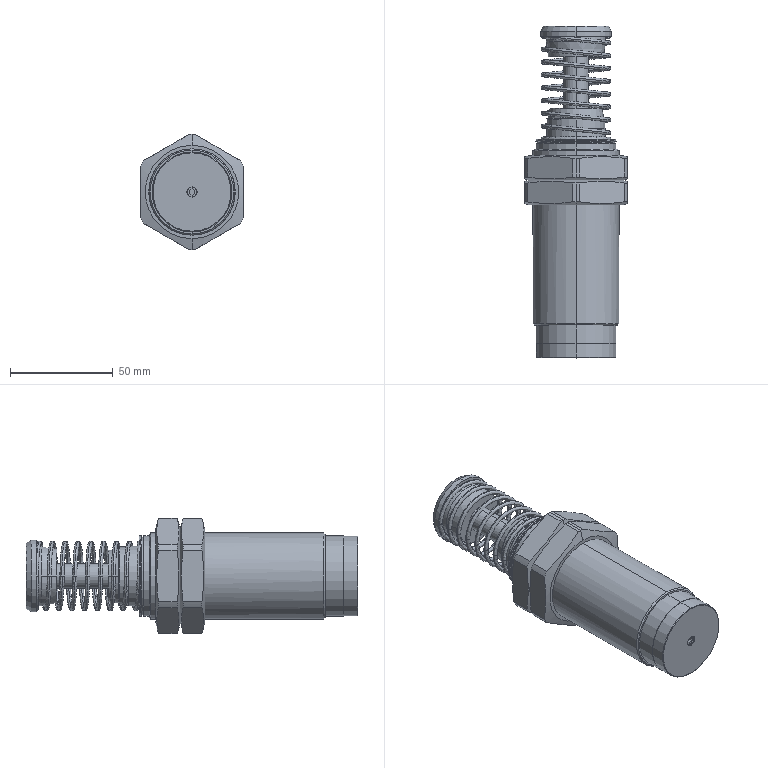Part | STEP file | ACJ4225F-AirTAC | 3 solids | 159 faces | box 50 x 161.5 x 56.022 mm | volume 187281 mm3 | spline 45 | cylinder 42 | plane 38 | cone 34 | commonest cylinder face diameters 56.022 x14 39 x6 28.8 x4 41.188 x4 4.459 x2 12 x2